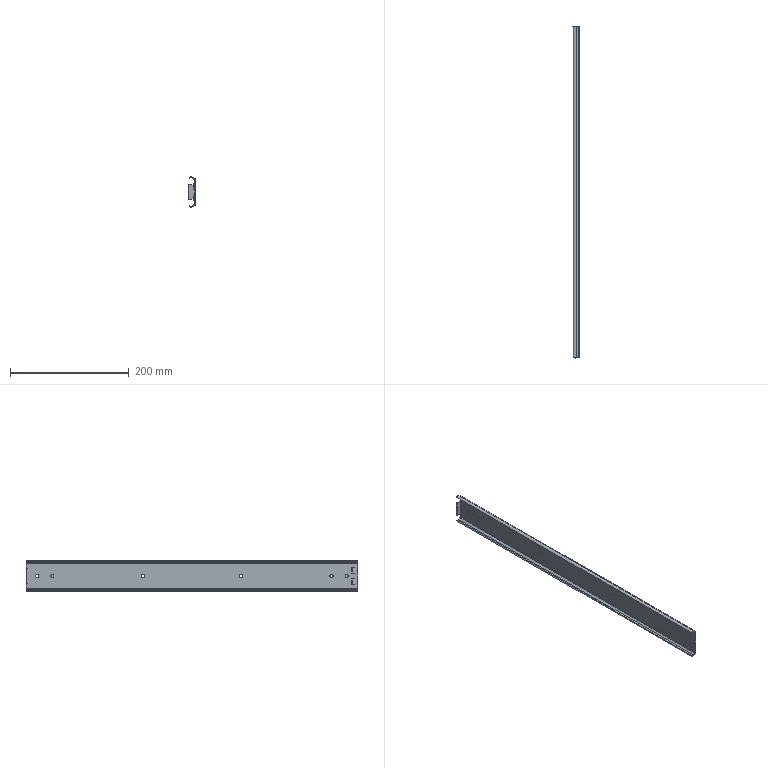Part | NX | features RAIL_5003_009_C-SRH51Y22 2 | 1 solid | 67 faces | box 11 x 558.8 x 51.5 mm | volume 56901 mm3 | plane 40 | cylinder 27 | commonest cylinder face diameters 4.5 x12 2 x4 1 x2 2.8 x2 3.8 x2 5.5 x2